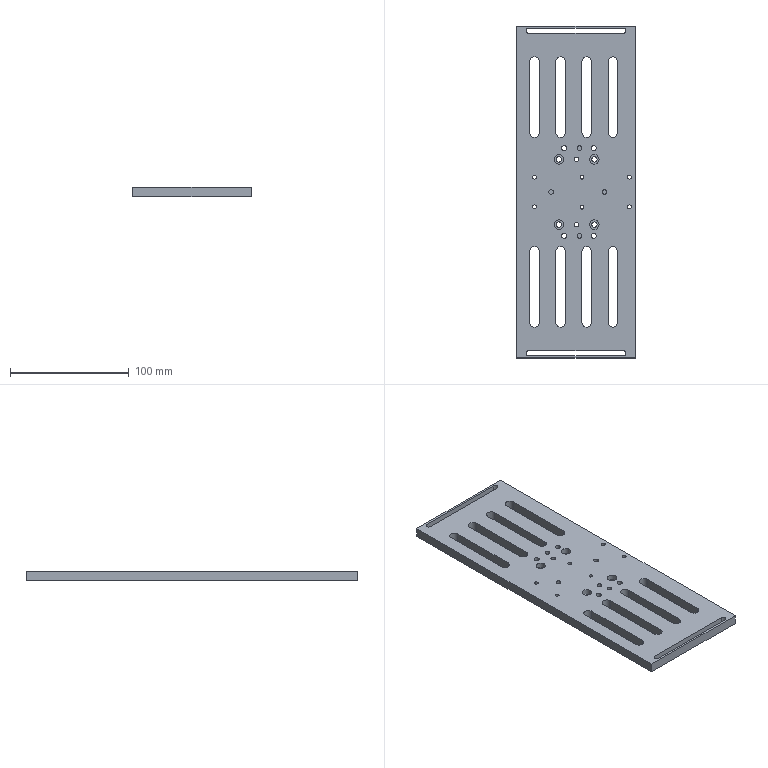Part | STEP file | SynoNew-0304-039 | 1 solid | 78 faces | box 100 x 280 x 8 mm | volume 182196 mm3 | cylinder 44 | plane 34 | commonest cylinder face diameters 8 x20 3.242 x6 4 x6 4.1 x4 4.2 x4 4.5 x4